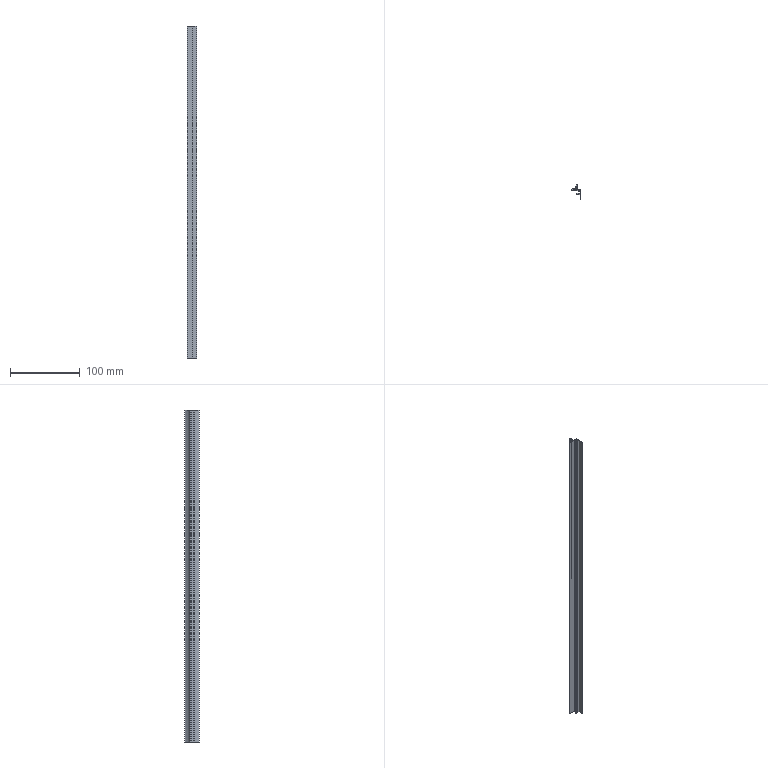Part | SolidWorks | features BaseBody 1, ICE 1, MoveFace 1 | 1 solid | 27 faces | box 14 x 20.3 x 476 mm | volume 24236 mm3 | plane 20 | cylinder 7 | commonest cylinder face diameters 0.387 x2 0.8 x2 0.4 x1 20 x1 22 x1
STEP:
#1=CARTESIAN_POINT('',(-5.304,-0.625,200.));
#2=VERTEX_POINT('',#1);
#3=CARTESIAN_POINT('',(-5.449,-0.8125,200.));
#4=VERTEX_POINT('',#3);
#5=CARTESIAN_POINT('',(-5.255,-0.8125,200.));
#6=DIRECTION('',(0.,0.,1.));
#7=DIRECTION('',(-1.,0.,0.));
#8=AXIS2_PLACEMENT_3D('',#5,#6,#7);
#9=CIRCLE('',#8,0.1937);
#10=EDGE_CURVE('',#2,#4,#9,.T.);
#11=ORIENTED_EDGE('',*,*,#10,.T.);
#12=CARTESIAN_POINT('',(-5.449,-0.8125,-276.));
#13=VERTEX_POINT('',#12);
#14=CARTESIAN_POINT('',(-5.449,-0.8125,230.));
#15=DIRECTION('',(0.,0.,-1.));
#16=VECTOR('',#15,1000.);
#17=LINE('',#14,#16);
#18=EDGE_CURVE('',#4,#13,#17,.T.);
#19=ORIENTED_EDGE('',*,*,#18,.T.);
#20=CARTESIAN_POINT('',(-5.304,-0.625,-276.));
#21=VERTEX_POINT('',#20);
#22=CARTESIAN_POINT('',(-5.255,-0.8125,-276.));
#23=DIRECTION('',(0.,0.,-1.));
#24=DIRECTION('',(1.,0.,0.));
#25=AXIS2_PLACEMENT_3D('',#22,#23,#24);
#26=CIRCLE('',#25,0.1937);
#27=EDGE_CURVE('',#13,#21,#26,.T.);
#28=ORIENTED_EDGE('',*,*,#27,.T.);
#29=CARTESIAN_POINT('',(-5.304,-0.625,230.));
#30=DIRECTION('',(0.,0.,-1.));
#31=VECTOR('',#30,1000.);
#32=LINE('',#29,#31);
#33=EDGE_CURVE('',#2,#21,#32,.T.);
#34=ORIENTED_EDGE('',*,*,#33,.F.);
#35=EDGE_LOOP('',(#11,#19,#28,#34));
#36=FACE_OUTER_BOUND('',#35,.T.);
#37=CARTESIAN_POINT('',(-5.255,-0.8125,230.));
#38=DIRECTION('',(0.,0.,-1.));
#39=DIRECTION('',(-1.,0.,0.));
#40=AXIS2_PLACEMENT_3D('',#37,#38,#39);
#41=CYLINDRICAL_SURFACE('',#40,0.1937);
#42=ADVANCED_FACE('',(#36),#41,.F.);
#43=CARTESIAN_POINT('',(5.,-1.,-276.));
#44=VERTEX_POINT('',#43);
#45=CARTESIAN_POINT('',(5.,-14.3,-276.));
#46=VERTEX_POINT('',#45);
#47=CARTESIAN_POINT('',(5.,29.623,-276.));
#48=DIRECTION('',(0.,-1.,0.));
#49=VECTOR('',#48,1000.);
#50=LINE('',#47,#49);
#51=EDGE_CURVE('',#44,#46,#50,.T.);
#52=ORIENTED_EDGE('',*,*,#51,.F.);
#53=CARTESIAN_POINT('',(5.,-1.,200.));
#54=VERTEX_POINT('',#53);
#55=CARTESIAN_POINT('',(5.,-1.,230.));
#56=DIRECTION('',(0.,0.,-1.));
#57=VECTOR('',#56,1000.);
#58=LINE('',#55,#57);
#59=EDGE_CURVE('',#54,#44,#58,.T.);
#60=ORIENTED_EDGE('',*,*,#59,.F.);
#61=CARTESIAN_POINT('',(5.,-14.3,200.));
#62=VERTEX_POINT('',#61);
#63=CARTESIAN_POINT('',(5.,-14.3,200.));
#64=DIRECTION('',(0.,1.,0.));
#65=VECTOR('',#64,1000.);
#66=LINE('',#63,#65);
#67=EDGE_CURVE('',#62,#54,#66,.T.);
#68=ORIENTED_EDGE('',*,*,#67,.F.);
#69=CARTESIAN_POINT('',(5.,-14.3,230.));
#70=DIRECTION('',(0.,0.,1.));
#71=VECTOR('',#70,1000.);
#72=LINE('',#69,#71);
#73=EDGE_CURVE('',#46,#62,#72,.T.);
#74=ORIENTED_EDGE('',*,*,#73,.F.);
#75=EDGE_LOOP('',(#52,#60,#68,#74));
#76=FACE_OUTER_BOUND('',#75,.T.);
#77=CARTESIAN_POINT('',(5.,-14.3,230.));
#78=DIRECTION('',(-1.,0.,0.));
#79=DIRECTION('',(0.,0.,1.));
#80=AXIS2_PLACEMENT_3D('',#77,#78,#79);
#81=PLANE('',#80);
#82=ADVANCED_FACE('',(#76),#81,.F.);
#83=CARTESIAN_POINT('',(-9.,-2.,-276.));
#84=VERTEX_POINT('',#83);
#85=CARTESIAN_POINT('',(-9.,-2.,200.));
#86=VERTEX_POINT('',#85);
#87=CARTESIAN_POINT('',(-9.,-2.,230.));
#88=DIRECTION('',(0.,0.,1.));
#89=VECTOR('',#88,1000.);
#90=LINE('',#87,#89);
#91=EDGE_CURVE('',#84,#86,#90,.T.);
#92=ORIENTED_EDGE('',*,*,#91,.F.);
#93=CARTESIAN_POINT('',(0.9,-2.,-276.));
#94=VERTEX_POINT('',#93);
#95=CARTESIAN_POINT('',(5.,-2.,-276.));
#96=DIRECTION('',(-1.,0.,0.));
#97=VECTOR('',#96,1000.);
#98=LINE('',#95,#97);
#99=EDGE_CURVE('',#94,#84,#98,.T.);
#100=ORIENTED_EDGE('',*,*,#99,.F.);
#101=CARTESIAN_POINT('',(0.9,-2.,200.));
#102=VERTEX_POINT('',#101);
#103=CARTESIAN_POINT('',(0.9,-2.,230.));
#104=DIRECTION('',(0.,0.,-1.));
#105=VECTOR('',#104,1000.);
#106=LINE('',#103,#105);
#107=EDGE_CURVE('',#102,#94,#106,.T.);
#108=ORIENTED_EDGE('',*,*,#107,.F.);
#109=CARTESIAN_POINT('',(5.,-2.,200.));
#110=DIRECTION('',(1.,0.,0.));
#111=VECTOR('',#110,1000.);
#112=LINE('',#109,#111);
#113=EDGE_CURVE('',#86,#102,#112,.T.);
#114=ORIENTED_EDGE('',*,*,#113,.F.);
#115=EDGE_LOOP('',(#92,#100,#108,#114));
#116=FACE_OUTER_BOUND('',#115,.T.);
#117=CARTESIAN_POINT('',(-9.,-2.,230.));
#118=DIRECTION('',(0.,1.,0.));
#119=DIRECTION('',(0.,0.,1.));
#120=AXIS2_PLACEMENT_3D('',#117,#118,#119);
#121=PLANE('',#120);
#122=ADVANCED_FACE('',(#116),#121,.F.);
#123=CARTESIAN_POINT('',(4.,-6.,200.));
#124=VERTEX_POINT('',#123);
#125=CARTESIAN_POINT('',(4.,-3.,200.));
#126=VERTEX_POINT('',#125);
#127=CARTESIAN_POINT('',(4.,29.623,200.));
#128=DIRECTION('',(0.,1.,0.));
#129=VECTOR('',#128,1000.);
#130=LINE('',#127,#129);
#131=EDGE_CURVE('',#124,#126,#130,.T.);
#132=ORIENTED_EDGE('',*,*,#131,.F.);
#133=CARTESIAN_POINT('',(1.,-6.,200.));
#134=VERTEX_POINT('',#133);
#135=CARTESIAN_POINT('',(5.,-6.,200.));
#136=DIRECTION('',(1.,0.,0.));
#137=VECTOR('',#136,1000.);
#138=LINE('',#135,#137);
#139=EDGE_CURVE('',#134,#124,#138,.T.);
#140=ORIENTED_EDGE('',*,*,#139,.F.);
#141=CARTESIAN_POINT('',(1.,-6.7,200.));
#142=VERTEX_POINT('',#141);
#143=CARTESIAN_POINT('',(1.,-6.,200.));
#144=DIRECTION('',(0.,-1.,0.));
#145=VECTOR('',#144,1000.);
#146=LINE('',#143,#145);
#147=EDGE_CURVE('',#134,#142,#146,.T.);
#148=ORIENTED_EDGE('',*,*,#147,.T.);
#149=CARTESIAN_POINT('',(-1.7,-6.7,200.));
#150=VERTEX_POINT('',#149);
#151=CARTESIAN_POINT('',(5.,-6.7,200.));
#152=DIRECTION('',(1.,0.,0.));
#153=VECTOR('',#152,1000.);
#154=LINE('',#151,#153);
#155=EDGE_CURVE('',#150,#142,#154,.T.);
#156=ORIENTED_EDGE('',*,*,#155,.F.);
#157=CARTESIAN_POINT('',(-1.7,-7.7,200.));
#158=VERTEX_POINT('',#157);
#159=CARTESIAN_POINT('',(-1.7,-6.7,200.));
#160=DIRECTION('',(0.,-1.,0.));
#161=VECTOR('',#160,1000.);
#162=LINE('',#159,#161);
#163=EDGE_CURVE('',#150,#158,#162,.T.);
#164=ORIENTED_EDGE('',*,*,#163,.T.);
#165=CARTESIAN_POINT('',(4.,-7.7,200.));
#166=VERTEX_POINT('',#165);
#167=CARTESIAN_POINT('',(5.,-7.7,200.));
#168=DIRECTION('',(-1.,0.,0.));
#169=VECTOR('',#168,1000.);
#170=LINE('',#167,#169);
#171=EDGE_CURVE('',#166,#158,#170,.T.);
#172=ORIENTED_EDGE('',*,*,#171,.F.);
#173=CARTESIAN_POINT('',(4.,-14.3,200.));
#174=VERTEX_POINT('',#173);
#175=CARTESIAN_POINT('',(4.,29.623,200.));
#176=DIRECTION('',(0.,1.,0.));
#177=VECTOR('',#176,1000.);
#178=LINE('',#175,#177);
#179=EDGE_CURVE('',#174,#166,#178,.T.);
#180=ORIENTED_EDGE('',*,*,#179,.F.);
#181=CARTESIAN_POINT('',(5.,-14.3,200.));
#182=DIRECTION('',(-1.,0.,0.));
#183=VECTOR('',#182,1000.);
#184=LINE('',#181,#183);
#185=EDGE_CURVE('',#62,#174,#184,.T.);
#186=ORIENTED_EDGE('',*,*,#185,.F.);
#187=ORIENTED_EDGE('',*,*,#67,.T.);
#188=CARTESIAN_POINT('',(-5.207,-1.,200.));
#189=VERTEX_POINT('',#188);
#190=CARTESIAN_POINT('',(5.,-1.,200.));
#191=DIRECTION('',(1.,0.,0.));
#192=VECTOR('',#191,1000.);
#193=LINE('',#190,#192);
#194=EDGE_CURVE('',#189,#54,#193,.T.);
#195=ORIENTED_EDGE('',*,*,#194,.F.);
#196=CARTESIAN_POINT('',(-5.255,-0.8125,200.));
#197=DIRECTION('',(0.,0.,1.));
#198=DIRECTION('',(-1.,0.,0.));
#199=AXIS2_PLACEMENT_3D('',#196,#197,#198);
#200=CIRCLE('',#199,0.1937);
#201=EDGE_CURVE('',#4,#189,#200,.T.);
#202=ORIENTED_EDGE('',*,*,#201,.F.);
#203=ORIENTED_EDGE('',*,*,#10,.F.);
#204=CARTESIAN_POINT('',(-1.368,3.063,200.));
#205=VERTEX_POINT('',#204);
#206=CARTESIAN_POINT('',(-10.628,9.,200.));
#207=DIRECTION('',(0.,0.,1.));
#208=DIRECTION('',(-1.,0.,0.));
#209=AXIS2_PLACEMENT_3D('',#206,#207,#208);
#210=CIRCLE('',#209,11.);
#211=EDGE_CURVE('',#2,#205,#210,.T.);
#212=ORIENTED_EDGE('',*,*,#211,.T.);
#213=CARTESIAN_POINT('',(-1.,2.955,200.));
#214=VERTEX_POINT('',#213);
#215=CARTESIAN_POINT('',(-1.2,2.955,200.));
#216=DIRECTION('',(0.,0.,1.));
#217=DIRECTION('',(-1.,0.,0.));
#218=AXIS2_PLACEMENT_3D('',#215,#216,#217);
#219=CIRCLE('',#218,0.2);
#220=EDGE_CURVE('',#214,#205,#219,.T.);
#221=ORIENTED_EDGE('',*,*,#220,.F.);
#222=CARTESIAN_POINT('',(-1.,1.5,200.));
#223=VERTEX_POINT('',#222);
#224=CARTESIAN_POINT('',(-1.,2.955,200.));
#225=DIRECTION('',(0.,1.,0.));
#226=VECTOR('',#225,1000.);
#227=LINE('',#224,#226);
#228=EDGE_CURVE('',#223,#214,#227,.T.);
#229=ORIENTED_EDGE('',*,*,#228,.F.);
#230=CARTESIAN_POINT('',(0.,1.5,200.));
#231=VERTEX_POINT('',#230);
#232=CARTESIAN_POINT('',(-1.,1.5,200.));
#233=DIRECTION('',(-1.,0.,0.));
#234=VECTOR('',#233,1000.);
#235=LINE('',#232,#234);
#236=EDGE_CURVE('',#231,#223,#235,.T.);
#237=ORIENTED_EDGE('',*,*,#236,.F.);
#238=CARTESIAN_POINT('',(0.,6.,200.));
#239=VERTEX_POINT('',#238);
#240=CARTESIAN_POINT('',(0.,1.5,200.));
#241=DIRECTION('',(0.,-1.,0.));
#242=VECTOR('',#241,1000.);
#243=LINE('',#240,#242);
#244=EDGE_CURVE('',#239,#231,#243,.T.);
#245=ORIENTED_EDGE('',*,*,#244,.F.);
#246=CARTESIAN_POINT('',(-0.8,6.,200.));
#247=VERTEX_POINT('',#246);
#248=CARTESIAN_POINT('',(0.,6.,200.));
#249=DIRECTION('',(1.,0.,0.));
#250=VECTOR('',#249,1000.);
#251=LINE('',#248,#250);
#252=EDGE_CURVE('',#247,#239,#251,.T.);
#253=ORIENTED_EDGE('',*,*,#252,.F.);
#254=CARTESIAN_POINT('',(-1.178,5.731,200.));
#255=VERTEX_POINT('',#254);
#256=CARTESIAN_POINT('',(-0.8,5.6,200.));
#257=DIRECTION('',(0.,0.,1.));
#258=DIRECTION('',(-1.,0.,0.));
#259=AXIS2_PLACEMENT_3D('',#256,#257,#258);
#260=CIRCLE('',#259,0.4);
#261=EDGE_CURVE('',#247,#255,#260,.T.);
#262=ORIENTED_EDGE('',*,*,#261,.T.);
#263=CARTESIAN_POINT('',(-8.678,-0.8077,200.));
#264=VERTEX_POINT('',#263);
#265=CARTESIAN_POINT('',(-10.628,9.,200.));
#266=DIRECTION('',(0.,0.,1.));
#267=DIRECTION('',(-1.,0.,0.));
#268=AXIS2_PLACEMENT_3D('',#265,#266,#267);
#269=CIRCLE('',#268,10.);
#270=EDGE_CURVE('',#264,#255,#269,.T.);
#271=ORIENTED_EDGE('',*,*,#270,.F.);
#272=CARTESIAN_POINT('',(-9.,-1.2,200.));
#273=VERTEX_POINT('',#272);
#274=CARTESIAN_POINT('',(-8.6,-1.2,200.));
#275=DIRECTION('',(0.,0.,1.));
#276=DIRECTION('',(-1.,0.,0.));
#277=AXIS2_PLACEMENT_3D('',#274,#275,#276);
#278=CIRCLE('',#277,0.4);
#279=EDGE_CURVE('',#264,#273,#278,.T.);
#280=ORIENTED_EDGE('',*,*,#279,.T.);
#281=CARTESIAN_POINT('',(-9.,8.,200.));
#282=DIRECTION('',(0.,-1.,0.));
#283=VECTOR('',#282,1000.);
#284=LINE('',#281,#283);
#285=EDGE_CURVE('',#273,#86,#284,.T.);
#286=ORIENTED_EDGE('',*,*,#285,.T.);
#287=ORIENTED_EDGE('',*,*,#113,.T.);
#288=CARTESIAN_POINT('',(0.9,-3.,200.));
#289=VERTEX_POINT('',#288);
#290=CARTESIAN_POINT('',(0.9,29.623,200.));
#291=DIRECTION('',(0.,1.,0.));
#292=VECTOR('',#291,1000.);
#293=LINE('',#290,#292);
#294=EDGE_CURVE('',#289,#102,#293,.T.);
#295=ORIENTED_EDGE('',*,*,#294,.F.);
#296=CARTESIAN_POINT('',(5.,-3.,200.));
#297=DIRECTION('',(-1.,0.,0.));
#298=VECTOR('',#297,1000.);
#299=LINE('',#296,#298);
#300=EDGE_CURVE('',#126,#289,#299,.T.);
#301=ORIENTED_EDGE('',*,*,#300,.F.);
#302=EDGE_LOOP('',(#132,#140,#148,#156,#164,#172,#180,#186,#187,#195,#202,#203,#212,#221,#229,#237,#245,#253,#262,#271,#280,#286,#287,#295,#301));
#303=FACE_OUTER_BOUND('',#302,.T.);
#304=CARTESIAN_POINT('',(5.,29.623,200.));
#305=DIRECTION('',(0.,0.,-1.));
#306=DIRECTION('',(-1.,0.,0.));
#307=AXIS2_PLACEMENT_3D('',#304,#305,#306);
#308=PLANE('',#307);
#309=ADVANCED_FACE('',(#303),#308,.F.);
#310=ORIENTED_EDGE('',*,*,#185,.T.);
#311=CARTESIAN_POINT('',(4.,-14.3,-276.));
#312=VERTEX_POINT('',#311);
#313=CARTESIAN_POINT('',(4.,-14.3,230.));
#314=DIRECTION('',(0.,0.,1.));
#315=VECTOR('',#314,1000.);
#316=LINE('',#313,#315);
#317=EDGE_CURVE('',#312,#174,#316,.T.);
#318=ORIENTED_EDGE('',*,*,#317,.F.);
#319=CARTESIAN_POINT('',(5.,-14.3,-276.));
#320=DIRECTION('',(-1.,0.,0.));
#321=VECTOR('',#320,1000.);
#322=LINE('',#319,#321);
#323=EDGE_CURVE('',#46,#312,#322,.T.);
#324=ORIENTED_EDGE('',*,*,#323,.F.);
#325=ORIENTED_EDGE('',*,*,#73,.T.);
#326=EDGE_LOOP('',(#310,#318,#324,#325));
#327=FACE_OUTER_BOUND('',#326,.T.);
#328=CARTESIAN_POINT('',(4.,-14.3,230.));
#329=DIRECTION('',(0.,1.,0.));
#330=DIRECTION('',(0.,0.,1.));
#331=AXIS2_PLACEMENT_3D('',#328,#329,#330);
#332=PLANE('',#331);
#333=ADVANCED_FACE('',(#327),#332,.F.);
#334=ORIENTED_EDGE('',*,*,#51,.T.);
#335=ORIENTED_EDGE('',*,*,#323,.T.);
#336=CARTESIAN_POINT('',(4.,-7.7,-276.));
#337=VERTEX_POINT('',#336);
#338=CARTESIAN_POINT('',(4.,-7.7,-276.));
#339=DIRECTION('',(0.,-1.,0.));
#340=VECTOR('',#339,1000.);
#341=LINE('',#338,#340);
#342=EDGE_CURVE('',#337,#312,#341,.T.);
#343=ORIENTED_EDGE('',*,*,#342,.F.);
#344=CARTESIAN_POINT('',(-1.7,-7.7,-276.));
#345=VERTEX_POINT('',#344);
#346=CARTESIAN_POINT('',(-1.7,-7.7,-276.));
#347=DIRECTION('',(1.,0.,0.));
#348=VECTOR('',#347,1000.);
#349=LINE('',#346,#348);
#350=EDGE_CURVE('',#345,#337,#349,.T.);
#351=ORIENTED_EDGE('',*,*,#350,.F.);
#352=CARTESIAN_POINT('',(-1.7,-6.7,-276.));
#353=VERTEX_POINT('',#352);
#354=CARTESIAN_POINT('',(-1.7,29.623,-276.));
#355=DIRECTION('',(0.,1.,0.));
#356=VECTOR('',#355,1000.);
#357=LINE('',#354,#356);
#358=EDGE_CURVE('',#345,#353,#357,.T.);
#359=ORIENTED_EDGE('',*,*,#358,.T.);
#360=CARTESIAN_POINT('',(1.,-6.7,-276.));
#361=VERTEX_POINT('',#360);
#362=CARTESIAN_POINT('',(1.,-6.7,-276.));
#363=DIRECTION('',(-1.,0.,0.));
#364=VECTOR('',#363,1000.);
#365=LINE('',#362,#364);
#366=EDGE_CURVE('',#361,#353,#365,.T.);
#367=ORIENTED_EDGE('',*,*,#366,.F.);
#368=CARTESIAN_POINT('',(1.,-6.,-276.));
#369=VERTEX_POINT('',#368);
#370=CARTESIAN_POINT('',(1.,29.623,-276.));
#371=DIRECTION('',(0.,1.,0.));
#372=VECTOR('',#371,1000.);
#373=LINE('',#370,#372);
#374=EDGE_CURVE('',#361,#369,#373,.T.);
#375=ORIENTED_EDGE('',*,*,#374,.T.);
#376=CARTESIAN_POINT('',(4.,-6.,-276.));
#377=VERTEX_POINT('',#376);
#378=CARTESIAN_POINT('',(4.,-6.,-276.));
#379=DIRECTION('',(-1.,0.,0.));
#380=VECTOR('',#379,1000.);
#381=LINE('',#378,#380);
#382=EDGE_CURVE('',#377,#369,#381,.T.);
#383=ORIENTED_EDGE('',*,*,#382,.F.);
#384=CARTESIAN_POINT('',(4.,-3.,-276.));
#385=VERTEX_POINT('',#384);
#386=CARTESIAN_POINT('',(4.,-3.,-276.));
#387=DIRECTION('',(0.,-1.,0.));
#388=VECTOR('',#387,1000.);
#389=LINE('',#386,#388);
#390=EDGE_CURVE('',#385,#377,#389,.T.);
#391=ORIENTED_EDGE('',*,*,#390,.F.);
#392=CARTESIAN_POINT('',(0.9,-3.,-276.));
#393=VERTEX_POINT('',#392);
#394=CARTESIAN_POINT('',(0.9,-3.,-276.));
#395=DIRECTION('',(1.,0.,0.));
#396=VECTOR('',#395,1000.);
#397=LINE('',#394,#396);
#398=EDGE_CURVE('',#393,#385,#397,.T.);
#399=ORIENTED_EDGE('',*,*,#398,.F.);
#400=CARTESIAN_POINT('',(0.9,-2.,-276.));
#401=DIRECTION('',(0.,-1.,0.));
#402=VECTOR('',#401,1000.);
#403=LINE('',#400,#402);
#404=EDGE_CURVE('',#94,#393,#403,.T.);
#405=ORIENTED_EDGE('',*,*,#404,.F.);
#406=ORIENTED_EDGE('',*,*,#99,.T.);
#407=CARTESIAN_POINT('',(-9.,-1.2,-276.));
#408=VERTEX_POINT('',#407);
#409=CARTESIAN_POINT('',(-9.,-1.2,-276.));
#410=DIRECTION('',(0.,-1.,0.));
#411=VECTOR('',#410,1000.);
#412=LINE('',#409,#411);
#413=EDGE_CURVE('',#408,#84,#412,.T.);
#414=ORIENTED_EDGE('',*,*,#413,.F.);
#415=CARTESIAN_POINT('',(-8.678,-0.8077,-276.));
#416=VERTEX_POINT('',#415);
#417=CARTESIAN_POINT('',(-8.6,-1.2,-276.));
#418=DIRECTION('',(0.,0.,-1.));
#419=DIRECTION('',(1.,0.,0.));
#420=AXIS2_PLACEMENT_3D('',#417,#418,#419);
#421=CIRCLE('',#420,0.4);
#422=EDGE_CURVE('',#408,#416,#421,.T.);
#423=ORIENTED_EDGE('',*,*,#422,.T.);
#424=CARTESIAN_POINT('',(-1.178,5.731,-276.));
#425=VERTEX_POINT('',#424);
#426=CARTESIAN_POINT('',(-10.628,9.,-276.));
#427=DIRECTION('',(0.,0.,-1.));
#428=DIRECTION('',(1.,0.,0.));
#429=AXIS2_PLACEMENT_3D('',#426,#427,#428);
#430=CIRCLE('',#429,10.);
#431=EDGE_CURVE('',#425,#416,#430,.T.);
#432=ORIENTED_EDGE('',*,*,#431,.F.);
#433=CARTESIAN_POINT('',(-0.8,6.,-276.));
#434=VERTEX_POINT('',#433);
#435=CARTESIAN_POINT('',(-0.8,5.6,-276.));
#436=DIRECTION('',(0.,0.,-1.));
#437=DIRECTION('',(1.,0.,0.));
#438=AXIS2_PLACEMENT_3D('',#435,#436,#437);
#439=CIRCLE('',#438,0.4);
#440=EDGE_CURVE('',#425,#434,#439,.T.);
#441=ORIENTED_EDGE('',*,*,#440,.T.);
#442=CARTESIAN_POINT('',(0.,6.,-276.));
#443=VERTEX_POINT('',#442);
#444=CARTESIAN_POINT('',(0.,6.,-276.));
#445=DIRECTION('',(-1.,0.,0.));
#446=VECTOR('',#445,1000.);
#447=LINE('',#444,#446);
#448=EDGE_CURVE('',#443,#434,#447,.T.);
#449=ORIENTED_EDGE('',*,*,#448,.F.);
#450=CARTESIAN_POINT('',(0.,1.5,-276.));
#451=VERTEX_POINT('',#450);
#452=CARTESIAN_POINT('',(0.,1.5,-276.));
#453=DIRECTION('',(0.,1.,0.));
#454=VECTOR('',#453,1000.);
#455=LINE('',#452,#454);
#456=EDGE_CURVE('',#451,#443,#455,.T.);
#457=ORIENTED_EDGE('',*,*,#456,.F.);
#458=CARTESIAN_POINT('',(-1.,1.5,-276.));
#459=VERTEX_POINT('',#458);
#460=CARTESIAN_POINT('',(-1.,1.5,-276.));
#461=DIRECTION('',(1.,0.,0.));
#462=VECTOR('',#461,1000.);
#463=LINE('',#460,#462);
#464=EDGE_CURVE('',#459,#451,#463,.T.);
#465=ORIENTED_EDGE('',*,*,#464,.F.);
#466=CARTESIAN_POINT('',(-1.,2.955,-276.));
#467=VERTEX_POINT('',#466);
#468=CARTESIAN_POINT('',(-1.,2.955,-276.));
#469=DIRECTION('',(0.,-1.,0.));
#470=VECTOR('',#469,1000.);
#471=LINE('',#468,#470);
#472=EDGE_CURVE('',#467,#459,#471,.T.);
#473=ORIENTED_EDGE('',*,*,#472,.F.);
#474=CARTESIAN_POINT('',(-1.368,3.063,-276.));
#475=VERTEX_POINT('',#474);
#476=CARTESIAN_POINT('',(-1.2,2.955,-276.));
#477=DIRECTION('',(0.,0.,-1.));
#478=DIRECTION('',(1.,0.,0.));
#479=AXIS2_PLACEMENT_3D('',#476,#477,#478);
#480=CIRCLE('',#479,0.2);
#481=EDGE_CURVE('',#475,#467,#480,.T.);
#482=ORIENTED_EDGE('',*,*,#481,.F.);
#483=CARTESIAN_POINT('',(-10.628,9.,-276.));
#484=DIRECTION('',(0.,0.,-1.));
#485=DIRECTION('',(1.,0.,0.));
#486=AXIS2_PLACEMENT_3D('',#483,#484,#485);
#487=CIRCLE('',#486,11.);
#488=EDGE_CURVE('',#475,#21,#487,.T.);
#489=ORIENTED_EDGE('',*,*,#488,.T.);
#490=ORIENTED_EDGE('',*,*,#27,.F.);
#491=CARTESIAN_POINT('',(-5.207,-1.,-276.));
#492=VERTEX_POINT('',#491);
#493=CARTESIAN_POINT('',(-5.255,-0.8125,-276.));
#494=DIRECTION('',(0.,0.,-1.));
#495=DIRECTION('',(1.,0.,0.));
#496=AXIS2_PLACEMENT_3D('',#493,#494,#495);
#497=CIRCLE('',#496,0.1937);
#498=EDGE_CURVE('',#492,#13,#497,.T.);
#499=ORIENTED_EDGE('',*,*,#498,.F.);
#500=CARTESIAN_POINT('',(5.,-1.,-276.));
#501=DIRECTION('',(-1.,0.,0.));
#502=VECTOR('',#501,1000.);
#503=LINE('',#500,#502);
#504=EDGE_CURVE('',#44,#492,#503,.T.);
#505=ORIENTED_EDGE('',*,*,#504,.F.);
#506=EDGE_LOOP('',(#334,#335,#343,#351,#359,#367,#375,#383,#391,#399,#405,#406,#414,#423,#432,#441,#449,#457,#465,#473,#482,#489,#490,#499,#505));
#507=FACE_OUTER_BOUND('',#506,.T.);
#508=CARTESIAN_POINT('',(5.,29.623,-276.));
#509=DIRECTION('',(0.,0.,1.));
#510=DIRECTION('',(1.,0.,0.));
#511=AXIS2_PLACEMENT_3D('',#508,#509,#510);
#512=PLANE('',#511);
#513=ADVANCED_FACE('',(#507),#512,.F.);
#514=ORIENTED_EDGE('',*,*,#59,.T.);
#515=ORIENTED_EDGE('',*,*,#504,.T.);
#516=CARTESIAN_POINT('',(-5.207,-1.,230.));
#517=DIRECTION('',(0.,0.,-1.));
#518=VECTOR('',#517,1000.);
#519=LINE('',#516,#518);
#520=EDGE_CURVE('',#189,#492,#519,.T.);
#521=ORIENTED_EDGE('',*,*,#520,.F.);
#522=ORIENTED_EDGE('',*,*,#194,.T.);
#523=EDGE_LOOP('',(#514,#515,#521,#522));
#524=FACE_OUTER_BOUND('',#523,.T.);
#525=CARTESIAN_POINT('',(5.,-1.,230.));
#526=DIRECTION('',(0.,-1.,0.));
#527=DIRECTION('',(0.,0.,-1.));
#528=AXIS2_PLACEMENT_3D('',#525,#526,#527);
#529=PLANE('',#528);
#530=ADVANCED_FACE('',(#524),#529,.F.);
#531=CARTESIAN_POINT('',(-9.,-1.2,230.));
#532=DIRECTION('',(0.,0.,1.));
#533=VECTOR('',#532,1000.);
#534=LINE('',#531,#533);
#535=EDGE_CURVE('',#408,#273,#534,.T.);
#536=ORIENTED_EDGE('',*,*,#535,.F.);
#537=ORIENTED_EDGE('',*,*,#413,.T.);
#538=ORIENTED_EDGE('',*,*,#91,.T.);
#539=ORIENTED_EDGE('',*,*,#285,.F.);
#540=EDGE_LOOP('',(#536,#537,#538,#539));
#541=FACE_OUTER_BOUND('',#540,.T.);
#542=CARTESIAN_POINT('',(-9.,-1.2,230.));
#543=DIRECTION('',(1.,0.,0.));
#544=DIRECTION('',(0.,0.,-1.));
#545=AXIS2_PLACEMENT_3D('',#542,#543,#544);
#546=PLANE('',#545);
#547=ADVANCED_FACE('',(#541),#546,.F.);
#548=ORIENTED_EDGE('',*,*,#294,.T.);
#549=ORIENTED_EDGE('',*,*,#107,.T.);
#550=ORIENTED_EDGE('',*,*,#404,.T.);
#551=CARTESIAN_POINT('',(0.9,-3.,230.));
#552=DIRECTION('',(0.,0.,-1.));
#553=VECTOR('',#552,1000.);
#554=LINE('',#551,#553);
#555=EDGE_CURVE('',#289,#393,#554,.T.);
#556=ORIENTED_EDGE('',*,*,#555,.F.);
#557=EDGE_LOOP('',(#548,#549,#550,#556));
#558=FACE_OUTER_BOUND('',#557,.T.);
#559=CARTESIAN_POINT('',(0.9,-2.,230.));
#560=DIRECTION('',(1.,0.,0.));
#561=DIRECTION('',(0.,0.,-1.));
#562=AXIS2_PLACEMENT_3D('',#559,#560,#561);
#563=PLANE('',#562);
#564=ADVANCED_FACE('',(#558),#563,.F.);
#565=ORIENTED_EDGE('',*,*,#300,.T.);
#566=ORIENTED_EDGE('',*,*,#555,.T.);
#567=ORIENTED_EDGE('',*,*,#398,.T.);
#568=CARTESIAN_POINT('',(4.,-3.,230.));
#569=DIRECTION('',(0.,0.,-1.));
#570=VECTOR('',#569,1000.);
#571=LINE('',#568,#570);
#572=EDGE_CURVE('',#126,#385,#571,.T.);
#573=ORIENTED_EDGE('',*,*,#572,.F.);
#574=EDGE_LOOP('',(#565,#566,#567,#573));
#575=FACE_OUTER_BOUND('',#574,.T.);
#576=CARTESIAN_POINT('',(0.9,-3.,230.));
#577=DIRECTION('',(0.,1.,0.));
#578=DIRECTION('',(0.,0.,1.));
#579=AXIS2_PLACEMENT_3D('',#576,#577,#578);
#580=PLANE('',#579);
#581=ADVANCED_FACE('',(#575),#580,.F.);
#582=ORIENTED_EDGE('',*,*,#131,.T.);
#583=ORIENTED_EDGE('',*,*,#572,.T.);
#584=ORIENTED_EDGE('',*,*,#390,.T.);
#585=CARTESIAN_POINT('',(4.,-6.,230.));
#586=DIRECTION('',(0.,0.,-1.));
#587=VECTOR('',#586,1000.);
#588=LINE('',#585,#587);
#589=EDGE_CURVE('',#124,#377,#588,.T.);
#590=ORIENTED_EDGE('',*,*,#589,.F.);
#591=EDGE_LOOP('',(#582,#583,#584,#590));
#592=FACE_OUTER_BOUND('',#591,.T.);
#593=CARTESIAN_POINT('',(4.,-3.,230.));
#594=DIRECTION('',(1.,0.,0.));
#595=DIRECTION('',(0.,0.,-1.));
#596=AXIS2_PLACEMENT_3D('',#593,#594,#595);
#597=PLANE('',#596);
#598=ADVANCED_FACE('',(#592),#597,.F.);
#599=ORIENTED_EDGE('',*,*,#139,.T.);
#600=ORIENTED_EDGE('',*,*,#589,.T.);
#601=ORIENTED_EDGE('',*,*,#382,.T.);
#602=CARTESIAN_POINT('',(1.,-6.,230.));
#603=DIRECTION('',(0.,0.,-1.));
#604=VECTOR('',#603,1000.);
#605=LINE('',#602,#604);
#606=EDGE_CURVE('',#134,#369,#605,.T.);
#607=ORIENTED_EDGE('',*,*,#606,.F.);
#608=EDGE_LOOP('',(#599,#600,#601,#607));
#609=FACE_OUTER_BOUND('',#608,.T.);
#610=CARTESIAN_POINT('',(4.,-6.,230.));
#611=DIRECTION('',(0.,-1.,0.));
#612=DIRECTION('',(0.,0.,-1.));
#613=AXIS2_PLACEMENT_3D('',#610,#611,#612);
#614=PLANE('',#613);
#615=ADVANCED_FACE('',(#609),#614,.F.);
#616=ORIENTED_EDGE('',*,*,#155,.T.);
#617=CARTESIAN_POINT('',(1.,-6.7,230.));
#618=DIRECTION('',(0.,0.,1.));
#619=VECTOR('',#618,1000.);
#620=LINE('',#617,#619);
#621=EDGE_CURVE('',#361,#142,#620,.T.);
#622=ORIENTED_EDGE('',*,*,#621,.F.);
#623=ORIENTED_EDGE('',*,*,#366,.T.);
#624=CARTESIAN_POINT('',(-1.7,-6.7,230.));
#625=DIRECTION('',(0.,0.,-1.));
#626=VECTOR('',#625,1000.);
#627=LINE('',#624,#626);
#628=EDGE_CURVE('',#150,#353,#627,.T.);
#629=ORIENTED_EDGE('',*,*,#628,.F.);
#630=EDGE_LOOP('',(#616,#622,#623,#629));
#631=FACE_OUTER_BOUND('',#630,.T.);
#632=CARTESIAN_POINT('',(1.,-6.7,230.));
#633=DIRECTION('',(0.,-1.,0.));
#634=DIRECTION('',(0.,0.,-1.));
#635=AXIS2_PLACEMENT_3D('',#632,#633,#634);
#636=PLANE('',#635);
#637=ADVANCED_FACE('',(#631),#636,.F.);
#638=ORIENTED_EDGE('',*,*,#171,.T.);
#639=CARTESIAN_POINT('',(-1.7,-7.7,230.));
#640=DIRECTION('',(0.,0.,1.));
#641=VECTOR('',#640,1000.);
#642=LINE('',#639,#641);
#643=EDGE_CURVE('',#345,#158,#642,.T.);
#644=ORIENTED_EDGE('',*,*,#643,.F.);
#645=ORIENTED_EDGE('',*,*,#350,.T.);
#646=CARTESIAN_POINT('',(4.,-7.7,230.));
#647=DIRECTION('',(0.,0.,-1.));
#648=VECTOR('',#647,1000.);
#649=LINE('',#646,#648);
#650=EDGE_CURVE('',#166,#337,#649,.T.);
#651=ORIENTED_EDGE('',*,*,#650,.F.);
#652=EDGE_LOOP('',(#638,#644,#645,#651));
#653=FACE_OUTER_BOUND('',#652,.T.);
#654=CARTESIAN_POINT('',(-1.7,-7.7,230.));
#655=DIRECTION('',(0.,1.,0.));
#656=DIRECTION('',(0.,0.,1.));
#657=AXIS2_PLACEMENT_3D('',#654,#655,#656);
#658=PLANE('',#657);
#659=ADVANCED_FACE('',(#653),#658,.F.);
#660=ORIENTED_EDGE('',*,*,#179,.T.);
#661=ORIENTED_EDGE('',*,*,#650,.T.);
#662=ORIENTED_EDGE('',*,*,#342,.T.);
#663=ORIENTED_EDGE('',*,*,#317,.T.);
#664=EDGE_LOOP('',(#660,#661,#662,#663));
#665=FACE_OUTER_BOUND('',#664,.T.);
#666=CARTESIAN_POINT('',(4.,-7.7,230.));
#667=DIRECTION('',(1.,0.,0.));
#668=DIRECTION('',(0.,0.,-1.));
#669=AXIS2_PLACEMENT_3D('',#666,#667,#668);
#670=PLANE('',#669);
#671=ADVANCED_FACE('',(#665),#670,.F.);
#672=ORIENTED_EDGE('',*,*,#18,.F.);
#673=ORIENTED_EDGE('',*,*,#201,.T.);
#674=ORIENTED_EDGE('',*,*,#520,.T.);
#675=ORIENTED_EDGE('',*,*,#498,.T.);
#676=EDGE_LOOP('',(#672,#673,#674,#675));
#677=FACE_OUTER_BOUND('',#676,.T.);
#678=CARTESIAN_POINT('',(-5.255,-0.8125,230.));
#679=DIRECTION('',(0.,0.,-1.));
#680=DIRECTION('',(-1.,0.,0.));
#681=AXIS2_PLACEMENT_3D('',#678,#679,#680);
#682=CYLINDRICAL_SURFACE('',#681,0.1937);
#683=ADVANCED_FACE('',(#677),#682,.F.);
#684=CARTESIAN_POINT('',(-1.,2.955,230.));
#685=DIRECTION('',(0.,0.,1.));
#686=VECTOR('',#685,1000.);
#687=LINE('',#684,#686);
#688=EDGE_CURVE('',#467,#214,#687,.T.);
#689=ORIENTED_EDGE('',*,*,#688,.F.);
#690=ORIENTED_EDGE('',*,*,#472,.T.);
#691=CARTESIAN_POINT('',(-1.,1.5,230.));
#692=DIRECTION('',(0.,0.,-1.));
#693=VECTOR('',#692,1000.);
#694=LINE('',#691,#693);
#695=EDGE_CURVE('',#223,#459,#694,.T.);
#696=ORIENTED_EDGE('',*,*,#695,.F.);
#697=ORIENTED_EDGE('',*,*,#228,.T.);
#698=EDGE_LOOP('',(#689,#690,#696,#697));
#699=FACE_OUTER_BOUND('',#698,.T.);
#700=CARTESIAN_POINT('',(-1.,2.955,230.));
#701=DIRECTION('',(1.,0.,0.));
#702=DIRECTION('',(0.,0.,-1.));
#703=AXIS2_PLACEMENT_3D('',#700,#701,#702);
#704=PLANE('',#703);
#705=ADVANCED_FACE('',(#699),#704,.F.);
#706=ORIENTED_EDGE('',*,*,#488,.F.);
#707=CARTESIAN_POINT('',(-1.368,3.063,230.));
#708=DIRECTION('',(0.,0.,1.));
#709=VECTOR('',#708,1000.);
#710=LINE('',#707,#709);
#711=EDGE_CURVE('',#475,#205,#710,.T.);
#712=ORIENTED_EDGE('',*,*,#711,.T.);
#713=ORIENTED_EDGE('',*,*,#211,.F.);
#714=ORIENTED_EDGE('',*,*,#33,.T.);
#715=EDGE_LOOP('',(#706,#712,#713,#714));
#716=FACE_OUTER_BOUND('',#715,.T.);
#717=CARTESIAN_POINT('',(-10.628,9.,230.));
#718=DIRECTION('',(0.,0.,-1.));
#719=DIRECTION('',(-1.,0.,0.));
#720=AXIS2_PLACEMENT_3D('',#717,#718,#719);
#721=CYLINDRICAL_SURFACE('',#720,11.);
#722=ADVANCED_FACE('',(#716),#721,.T.);
#723=CARTESIAN_POINT('',(-1.178,5.731,230.));
#724=DIRECTION('',(0.,0.,1.));
#725=VECTOR('',#724,1000.);
#726=LINE('',#723,#725);
#727=EDGE_CURVE('',#425,#255,#726,.T.);
#728=ORIENTED_EDGE('',*,*,#727,.F.);
#729=ORIENTED_EDGE('',*,*,#431,.T.);
#730=CARTESIAN_POINT('',(-8.678,-0.8077,230.));
#731=DIRECTION('',(0.,0.,-1.));
#732=VECTOR('',#731,1000.);
#733=LINE('',#730,#732);
#734=EDGE_CURVE('',#264,#416,#733,.T.);
#735=ORIENTED_EDGE('',*,*,#734,.F.);
#736=ORIENTED_EDGE('',*,*,#270,.T.);
#737=EDGE_LOOP('',(#728,#729,#735,#736));
#738=FACE_OUTER_BOUND('',#737,.T.);
#739=CARTESIAN_POINT('',(-10.628,9.,230.));
#740=DIRECTION('',(0.,0.,-1.));
#741=DIRECTION('',(-1.,0.,0.));
#742=AXIS2_PLACEMENT_3D('',#739,#740,#741);
#743=CYLINDRICAL_SURFACE('',#742,10.);
#744=ADVANCED_FACE('',(#738),#743,.F.);
#745=CARTESIAN_POINT('',(0.,1.5,230.));
#746=DIRECTION('',(0.,0.,1.));
#747=VECTOR('',#746,1000.);
#748=LINE('',#745,#747);
#749=EDGE_CURVE('',#451,#231,#748,.T.);
#750=ORIENTED_EDGE('',*,*,#749,.F.);
#751=ORIENTED_EDGE('',*,*,#456,.T.);
#752=CARTESIAN_POINT('',(0.,6.,230.));
#753=DIRECTION('',(0.,0.,-1.));
#754=VECTOR('',#753,1000.);
#755=LINE('',#752,#754);
#756=EDGE_CURVE('',#239,#443,#755,.T.);
#757=ORIENTED_EDGE('',*,*,#756,.F.);
#758=ORIENTED_EDGE('',*,*,#244,.T.);
#759=EDGE_LOOP('',(#750,#751,#757,#758));
#760=FACE_OUTER_BOUND('',#759,.T.);
#761=CARTESIAN_POINT('',(0.,1.5,230.));
#762=DIRECTION('',(-1.,0.,0.));
#763=DIRECTION('',(0.,0.,1.));
#764=AXIS2_PLACEMENT_3D('',#761,#762,#763);
#765=PLANE('',#764);
#766=ADVANCED_FACE('',(#760),#765,.F.);
#767=ORIENTED_EDGE('',*,*,#422,.F.);
#768=ORIENTED_EDGE('',*,*,#535,.T.);
#769=ORIENTED_EDGE('',*,*,#279,.F.);
#770=ORIENTED_EDGE('',*,*,#734,.T.);
#771=EDGE_LOOP('',(#767,#768,#769,#770));
#772=FACE_OUTER_BOUND('',#771,.T.);
#773=CARTESIAN_POINT('',(-8.6,-1.2,230.));
#774=DIRECTION('',(0.,0.,-1.));
#775=DIRECTION('',(-1.,0.,0.));
#776=AXIS2_PLACEMENT_3D('',#773,#774,#775);
#777=CYLINDRICAL_SURFACE('',#776,0.4);
#778=ADVANCED_FACE('',(#772),#777,.T.);
#779=ORIENTED_EDGE('',*,*,#147,.F.);
#780=ORIENTED_EDGE('',*,*,#606,.T.);
#781=ORIENTED_EDGE('',*,*,#374,.F.);
#782=ORIENTED_EDGE('',*,*,#621,.T.);
#783=EDGE_LOOP('',(#779,#780,#781,#782));
#784=FACE_OUTER_BOUND('',#783,.T.);
#785=CARTESIAN_POINT('',(1.,-6.,230.));
#786=DIRECTION('',(1.,0.,0.));
#787=DIRECTION('',(0.,0.,-1.));
#788=AXIS2_PLACEMENT_3D('',#785,#786,#787);
#789=PLANE('',#788);
#790=ADVANCED_FACE('',(#784),#789,.F.);
#791=ORIENTED_EDGE('',*,*,#163,.F.);
#792=ORIENTED_EDGE('',*,*,#628,.T.);
#793=ORIENTED_EDGE('',*,*,#358,.F.);
#794=ORIENTED_EDGE('',*,*,#643,.T.);
#795=EDGE_LOOP('',(#791,#792,#793,#794));
#796=FACE_OUTER_BOUND('',#795,.T.);
#797=CARTESIAN_POINT('',(-1.7,-6.7,230.));
#798=DIRECTION('',(1.,0.,0.));
#799=DIRECTION('',(0.,0.,-1.));
#800=AXIS2_PLACEMENT_3D('',#797,#798,#799);
#801=PLANE('',#800);
#802=ADVANCED_FACE('',(#796),#801,.F.);
#803=ORIENTED_EDGE('',*,*,#711,.F.);
#804=ORIENTED_EDGE('',*,*,#481,.T.);
#805=ORIENTED_EDGE('',*,*,#688,.T.);
#806=ORIENTED_EDGE('',*,*,#220,.T.);
#807=EDGE_LOOP('',(#803,#804,#805,#806));
#808=FACE_OUTER_BOUND('',#807,.T.);
#809=CARTESIAN_POINT('',(-1.2,2.955,230.));
#810=DIRECTION('',(0.,0.,-1.));
#811=DIRECTION('',(-1.,0.,0.));
#812=AXIS2_PLACEMENT_3D('',#809,#810,#811);
#813=CYLINDRICAL_SURFACE('',#812,0.2);
#814=ADVANCED_FACE('',(#808),#813,.F.);
#815=ORIENTED_EDGE('',*,*,#695,.T.);
#816=ORIENTED_EDGE('',*,*,#464,.T.);
#817=ORIENTED_EDGE('',*,*,#749,.T.);
#818=ORIENTED_EDGE('',*,*,#236,.T.);
#819=EDGE_LOOP('',(#815,#816,#817,#818));
#820=FACE_OUTER_BOUND('',#819,.T.);
#821=CARTESIAN_POINT('',(-1.,1.5,230.));
#822=DIRECTION('',(0.,1.,0.));
#823=DIRECTION('',(0.,0.,1.));
#824=AXIS2_PLACEMENT_3D('',#821,#822,#823);
#825=PLANE('',#824);
#826=ADVANCED_FACE('',(#820),#825,.F.);
#827=ORIENTED_EDGE('',*,*,#440,.F.);
#828=ORIENTED_EDGE('',*,*,#727,.T.);
#829=ORIENTED_EDGE('',*,*,#261,.F.);
#830=CARTESIAN_POINT('',(-0.8,6.,230.));
#831=DIRECTION('',(0.,0.,-1.));
#832=VECTOR('',#831,1000.);
#833=LINE('',#830,#832);
#834=EDGE_CURVE('',#247,#434,#833,.T.);
#835=ORIENTED_EDGE('',*,*,#834,.T.);
#836=EDGE_LOOP('',(#827,#828,#829,#835));
#837=FACE_OUTER_BOUND('',#836,.T.);
#838=CARTESIAN_POINT('',(-0.8,5.6,230.));
#839=DIRECTION('',(0.,0.,-1.));
#840=DIRECTION('',(-1.,0.,0.));
#841=AXIS2_PLACEMENT_3D('',#838,#839,#840);
#842=CYLINDRICAL_SURFACE('',#841,0.4);
#843=ADVANCED_FACE('',(#837),#842,.T.);
#844=ORIENTED_EDGE('',*,*,#756,.T.);
#845=ORIENTED_EDGE('',*,*,#448,.T.);
#846=ORIENTED_EDGE('',*,*,#834,.F.);
#847=ORIENTED_EDGE('',*,*,#252,.T.);
#848=EDGE_LOOP('',(#844,#845,#846,#847));
#849=FACE_OUTER_BOUND('',#848,.T.);
#850=CARTESIAN_POINT('',(0.,6.,230.));
#851=DIRECTION('',(0.,-1.,0.));
#852=DIRECTION('',(0.,0.,-1.));
#853=AXIS2_PLACEMENT_3D('',#850,#851,#852);
#854=PLANE('',#853);
#855=ADVANCED_FACE('',(#849),#854,.F.);
#856=CLOSED_SHELL('',(#42,#82,#122,#309,#333,#513,#530,#547,#564,#581,#598,#615,#637,#659,#671,#683,#705,#722,#744,#766,#778,#790,#802,#814,#826,#843,#855));
#857=MANIFOLD_SOLID_BREP('',#856);
#858=CARTESIAN_POINT('',(0.,0.,0.));
#859=DIRECTION('',(0.,0.,1.));
#860=DIRECTION('',(1.,0.,0.));
#861=AXIS2_PLACEMENT_3D('',#858,#859,#860);
#862=(LENGTH_UNIT()NAMED_UNIT(*)SI_UNIT(.MILLI.,.METRE.));
#863=UNCERTAINTY_MEASURE_WITH_UNIT(LENGTH_MEASURE(0.00001),#862,'','');
#864=(NAMED_UNIT(*)PLANE_ANGLE_UNIT()SI_UNIT($,.RADIAN.));
#865=(NAMED_UNIT(*)SI_UNIT($,.STERADIAN.)SOLID_ANGLE_UNIT());
#866=(GEOMETRIC_REPRESENTATION_CONTEXT(3)GLOBAL_UNCERTAINTY_ASSIGNED_CONTEXT((#863))GLOBAL_UNIT_ASSIGNED_CONTEXT((#862,#864,#865))REPRESENTATION_CONTEXT('',''));
#867=ADVANCED_BREP_SHAPE_REPRESENTATION('',(#857,#861),#866);